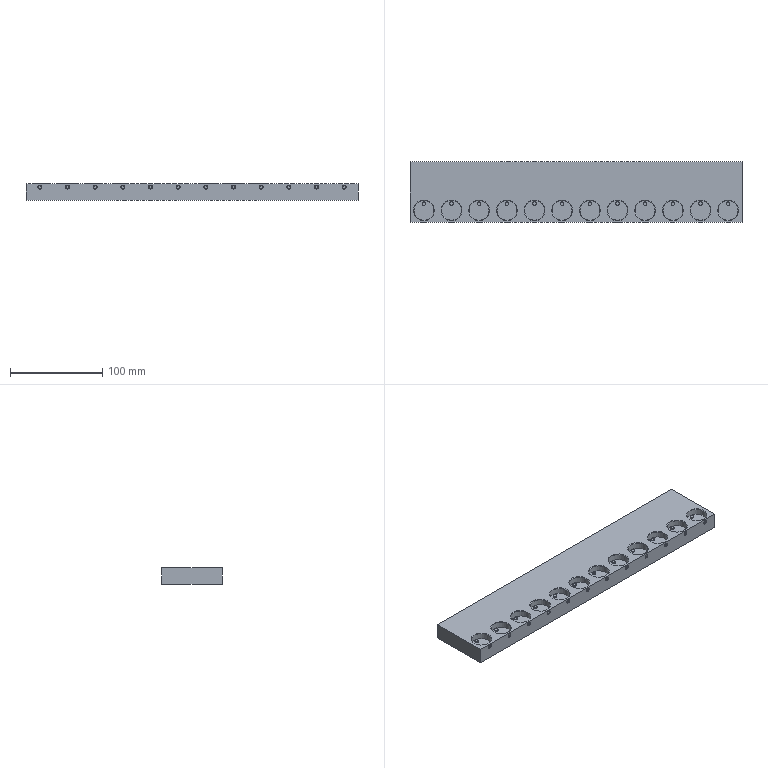Part | 1 solid | 102 faces | box 360 x 66 x 17.6 mm | volume 387469 mm3 | cylinder 36 | cone 36 | plane 30 | commonest cylinder face diameters 3.3 x12 3.91 x12 21.5 x12